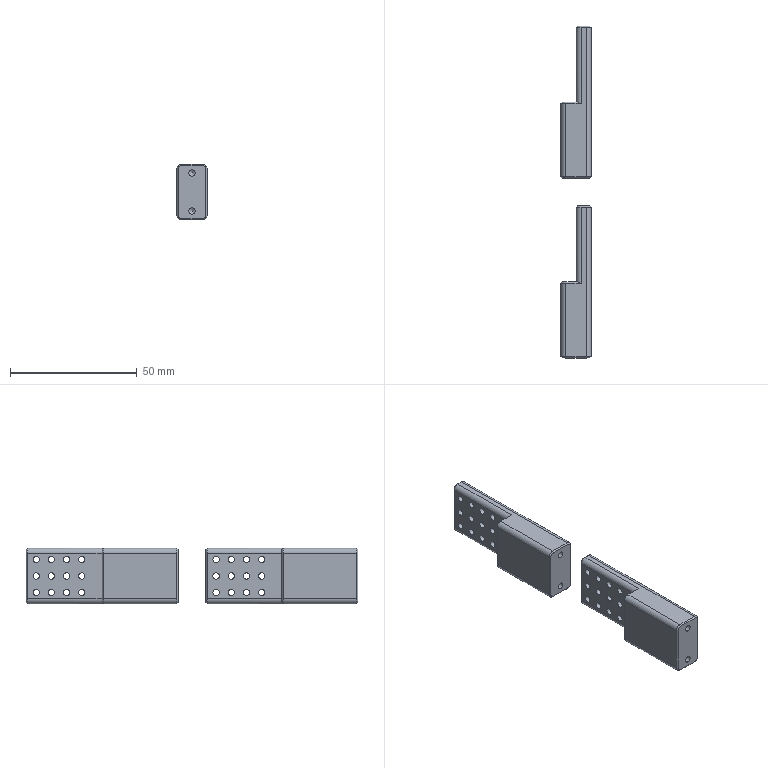Part | 2 solids | 102 faces | box 12 x 131 x 22 mm | volume 22452 mm3 | cylinder 40 | plane 38 | cone 24 | commonest cylinder face diameters 2.5 x28 4 x12